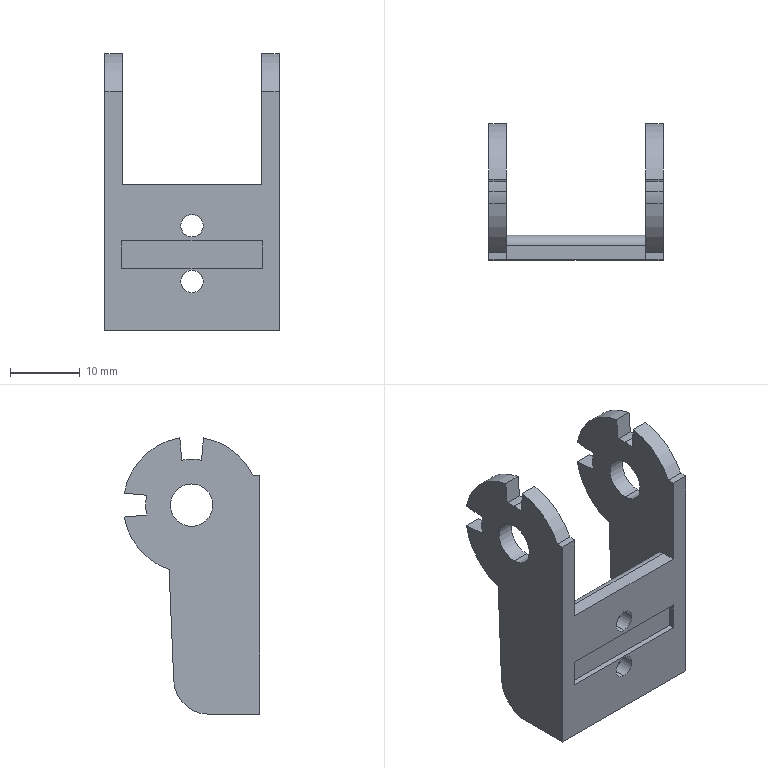Part | STEP file | _VED02-F15-001.stp | 1 solid | 52 faces | box 25 x 19.468 x 39.663 mm | volume 3938 mm3 | plane 25 | cylinder 23 | cone 4 | commonest cylinder face diameters 13.178 x6 3.2 x4 6.1 x4 19.618 x4 10 x2 19.616 x2